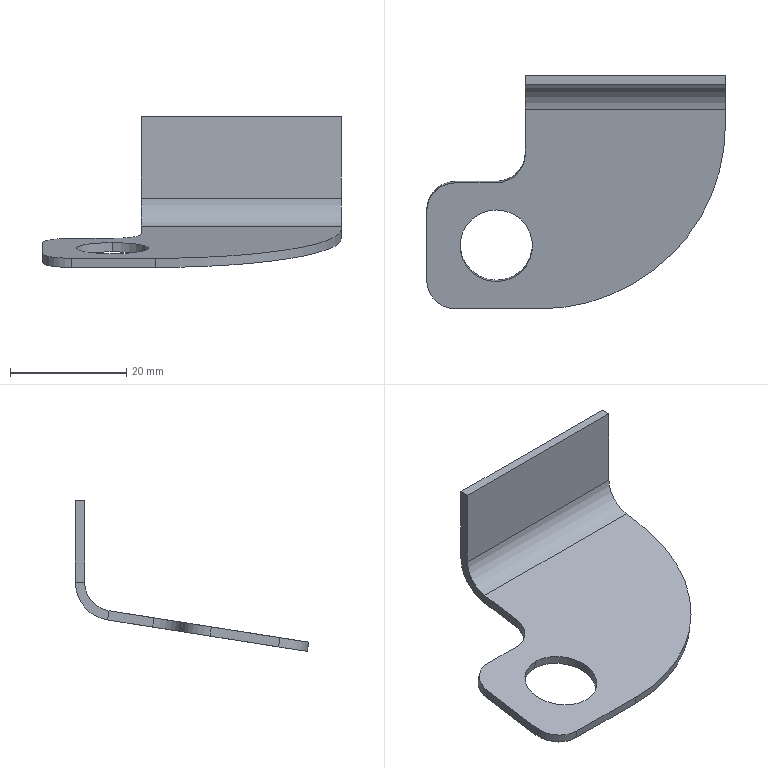Part | SolidWorks | features Fillet 2, ICE 2, FlatPattern 1, SMBaseFlange 1, SheetMetal 1 | 1 solid | 22 faces | box 51.5 x 40.249 x 26 mm | volume 3195 mm3 | plane 14 | cylinder 8 | commonest cylinder face diameters 10 x4 12.5 x2 13.2 x1 64 x1
STEP:
#1=CARTESIAN_POINT('',(-39.5,-23.209,-21.736));
#2=VERTEX_POINT('',#1);
#3=CARTESIAN_POINT('',(-39.5,-35.557,-23.68));
#4=VERTEX_POINT('',#3);
#5=CARTESIAN_POINT('',(-39.5,-29.383,-22.708));
#6=DIRECTION('',(0.,-0.1556,0.9878));
#7=DIRECTION('',(0.,-0.9878,-0.1556));
#8=AXIS2_PLACEMENT_3D('',#5,#6,#7);
#9=CIRCLE('',#8,6.25);
#10=EDGE_CURVE('',#2,#4,#9,.T.);
#11=ORIENTED_EDGE('',*,*,#10,.T.);
#12=CARTESIAN_POINT('',(-39.5,-35.308,-25.261));
#13=VERTEX_POINT('',#12);
#14=CARTESIAN_POINT('',(-39.5,-36.864,-15.383));
#15=DIRECTION('',(0.,0.1556,-0.9878));
#16=VECTOR('',#15,1000.);
#17=LINE('',#14,#16);
#18=EDGE_CURVE('',#4,#13,#17,.T.);
#19=ORIENTED_EDGE('',*,*,#18,.T.);
#20=CARTESIAN_POINT('',(-39.5,-22.96,-23.316));
#21=VERTEX_POINT('',#20);
#22=CARTESIAN_POINT('',(-39.5,-29.134,-24.289));
#23=DIRECTION('',(0.,0.1556,-0.9878));
#24=DIRECTION('',(0.,0.9878,0.1556));
#25=AXIS2_PLACEMENT_3D('',#22,#23,#24);
#26=CIRCLE('',#25,6.25);
#27=EDGE_CURVE('',#13,#21,#26,.T.);
#28=ORIENTED_EDGE('',*,*,#27,.T.);
#29=CARTESIAN_POINT('',(-39.5,-24.516,-13.438));
#30=DIRECTION('',(0.,0.1556,-0.9878));
#31=VECTOR('',#30,1000.);
#32=LINE('',#29,#31);
#33=EDGE_CURVE('',#2,#21,#32,.T.);
#34=ORIENTED_EDGE('',*,*,#33,.F.);
#35=EDGE_LOOP('',(#11,#19,#28,#34));
#36=FACE_OUTER_BOUND('',#35,.T.);
#37=CARTESIAN_POINT('',(-39.5,-30.69,-14.41));
#38=DIRECTION('',(0.,0.1556,-0.9878));
#39=DIRECTION('',(0.,0.9878,0.1556));
#40=AXIS2_PLACEMENT_3D('',#37,#38,#39);
#41=CYLINDRICAL_SURFACE('',#40,6.25);
#42=ADVANCED_FACE('',(#36),#41,.F.);
#43=CARTESIAN_POINT('',(-34.5,0.,-14.058));
#44=VERTEX_POINT('',#43);
#45=CARTESIAN_POINT('',(-34.5,0.,0.));
#46=VERTEX_POINT('',#45);
#47=CARTESIAN_POINT('',(-34.5,0.,0.));
#48=DIRECTION('',(0.,0.,1.));
#49=VECTOR('',#48,1000.);
#50=LINE('',#47,#49);
#51=EDGE_CURVE('',#44,#46,#50,.T.);
#52=ORIENTED_EDGE('',*,*,#51,.F.);
#53=CARTESIAN_POINT('',(-34.5,-1.6,-14.058));
#54=VERTEX_POINT('',#53);
#55=CARTESIAN_POINT('',(-34.5,0.,-14.058));
#56=DIRECTION('',(0.,-1.,0.));
#57=VECTOR('',#56,1000.);
#58=LINE('',#55,#57);
#59=EDGE_CURVE('',#44,#54,#58,.T.);
#60=ORIENTED_EDGE('',*,*,#59,.T.);
#61=CARTESIAN_POINT('',(-34.5,-1.6,0.));
#62=VERTEX_POINT('',#61);
#63=CARTESIAN_POINT('',(-34.5,-1.6,0.));
#64=DIRECTION('',(0.,0.,1.));
#65=VECTOR('',#64,1000.);
#66=LINE('',#63,#65);
#67=EDGE_CURVE('',#54,#62,#66,.T.);
#68=ORIENTED_EDGE('',*,*,#67,.T.);
#69=CARTESIAN_POINT('',(-34.5,-1.6,0.));
#70=DIRECTION('',(0.,-1.,0.));
#71=VECTOR('',#70,1000.);
#72=LINE('',#69,#71);
#73=EDGE_CURVE('',#46,#62,#72,.T.);
#74=ORIENTED_EDGE('',*,*,#73,.F.);
#75=EDGE_LOOP('',(#52,#60,#68,#74));
#76=FACE_OUTER_BOUND('',#75,.T.);
#77=CARTESIAN_POINT('',(-34.5,1.435,-115.54));
#78=DIRECTION('',(1.,0.,0.));
#79=DIRECTION('',(0.,0.,-1.));
#80=AXIS2_PLACEMENT_3D('',#77,#78,#79);
#81=PLANE('',#80);
#82=ADVANCED_FACE('',(#76),#81,.F.);
#83=CARTESIAN_POINT('',(-34.5,-13.578,-20.219));
#84=VERTEX_POINT('',#83);
#85=CARTESIAN_POINT('',(-34.5,-5.822,-18.997));
#86=VERTEX_POINT('',#85);
#87=CARTESIAN_POINT('',(-34.5,-0.2489,-18.119));
#88=DIRECTION('',(0.,0.9878,0.1556));
#89=VECTOR('',#88,1000.);
#90=LINE('',#87,#89);
#91=EDGE_CURVE('',#84,#86,#90,.T.);
#92=ORIENTED_EDGE('',*,*,#91,.T.);
#93=CARTESIAN_POINT('',(-34.5,-5.573,-20.578));
#94=VERTEX_POINT('',#93);
#95=CARTESIAN_POINT('',(-34.5,-5.822,-18.997));
#96=DIRECTION('',(0.,0.1556,-0.9878));
#97=VECTOR('',#96,1000.);
#98=LINE('',#95,#97);
#99=EDGE_CURVE('',#86,#94,#98,.T.);
#100=ORIENTED_EDGE('',*,*,#99,.T.);
#101=CARTESIAN_POINT('',(-34.5,-13.329,-21.799));
#102=VERTEX_POINT('',#101);
#103=CARTESIAN_POINT('',(-34.5,0.,-19.7));
#104=DIRECTION('',(0.,0.9878,0.1556));
#105=VECTOR('',#104,1000.);
#106=LINE('',#103,#105);
#107=EDGE_CURVE('',#102,#94,#106,.T.);
#108=ORIENTED_EDGE('',*,*,#107,.F.);
#109=CARTESIAN_POINT('',(-34.5,1.435,-115.54));
#110=DIRECTION('',(0.,-0.1556,0.9878));
#111=VECTOR('',#110,1000.);
#112=LINE('',#109,#111);
#113=EDGE_CURVE('',#102,#84,#112,.T.);
#114=ORIENTED_EDGE('',*,*,#113,.T.);
#115=EDGE_LOOP('',(#92,#100,#108,#114));
#116=FACE_OUTER_BOUND('',#115,.T.);
#117=CARTESIAN_POINT('',(-34.5,1.435,-115.54));
#118=DIRECTION('',(1.,0.,0.));
#119=DIRECTION('',(0.,0.,-1.));
#120=AXIS2_PLACEMENT_3D('',#117,#118,#119);
#121=PLANE('',#120);
#122=ADVANCED_FACE('',(#116),#121,.F.);
#123=CARTESIAN_POINT('',(0.,-5.573,-20.578));
#124=VERTEX_POINT('',#123);
#125=CARTESIAN_POINT('',(0.,-5.822,-18.997));
#126=VERTEX_POINT('',#125);
#127=CARTESIAN_POINT('',(0.,-5.573,-20.578));
#128=DIRECTION('',(0.,-0.1556,0.9878));
#129=VECTOR('',#128,1000.);
#130=LINE('',#127,#129);
#131=EDGE_CURVE('',#124,#126,#130,.T.);
#132=ORIENTED_EDGE('',*,*,#131,.F.);
#133=CARTESIAN_POINT('',(0.,0.,-14.058));
#134=VERTEX_POINT('',#133);
#135=CARTESIAN_POINT('',(0.,-6.6,-14.058));
#136=DIRECTION('',(-1.,0.,0.));
#137=DIRECTION('',(0.,0.,-1.));
#138=AXIS2_PLACEMENT_3D('',#135,#136,#137);
#139=CIRCLE('',#138,6.6);
#140=EDGE_CURVE('',#134,#124,#139,.T.);
#141=ORIENTED_EDGE('',*,*,#140,.F.);
#142=CARTESIAN_POINT('',(0.,-1.6,-14.058));
#143=VERTEX_POINT('',#142);
#144=CARTESIAN_POINT('',(0.,-1.6,-14.058));
#145=DIRECTION('',(0.,1.,0.));
#146=VECTOR('',#145,1000.);
#147=LINE('',#144,#146);
#148=EDGE_CURVE('',#143,#134,#147,.T.);
#149=ORIENTED_EDGE('',*,*,#148,.F.);
#150=CARTESIAN_POINT('',(0.,-6.6,-14.058));
#151=DIRECTION('',(-1.,0.,0.));
#152=DIRECTION('',(0.,0.,-1.));
#153=AXIS2_PLACEMENT_3D('',#150,#151,#152);
#154=CIRCLE('',#153,5.);
#155=EDGE_CURVE('',#143,#126,#154,.T.);
#156=ORIENTED_EDGE('',*,*,#155,.T.);
#157=EDGE_LOOP('',(#132,#141,#149,#156));
#158=FACE_OUTER_BOUND('',#157,.T.);
#159=CARTESIAN_POINT('',(0.,-5.573,-20.578));
#160=DIRECTION('',(1.,0.,0.));
#161=DIRECTION('',(0.,0.,-1.));
#162=AXIS2_PLACEMENT_3D('',#159,#160,#161);
#163=PLANE('',#162);
#164=ADVANCED_FACE('',(#158),#163,.T.);
#165=CARTESIAN_POINT('',(0.,-8.639,-19.441));
#166=VERTEX_POINT('',#165);
#167=CARTESIAN_POINT('',(0.,-0.2489,-18.119));
#168=DIRECTION('',(0.,-0.9878,-0.1556));
#169=VECTOR('',#168,1000.);
#170=LINE('',#167,#169);
#171=EDGE_CURVE('',#126,#166,#170,.T.);
#172=ORIENTED_EDGE('',*,*,#171,.T.);
#173=CARTESIAN_POINT('',(0.,-8.39,-21.021));
#174=VERTEX_POINT('',#173);
#175=CARTESIAN_POINT('',(0.,-8.39,-21.021));
#176=DIRECTION('',(0.,0.1556,-0.9878));
#177=VECTOR('',#176,1000.);
#178=LINE('',#175,#177);
#179=EDGE_CURVE('',#166,#174,#178,.T.);
#180=ORIENTED_EDGE('',*,*,#179,.T.);
#181=CARTESIAN_POINT('',(0.,0.,-19.7));
#182=DIRECTION('',(0.,-0.9878,-0.1556));
#183=VECTOR('',#182,1000.);
#184=LINE('',#181,#183);
#185=EDGE_CURVE('',#124,#174,#184,.T.);
#186=ORIENTED_EDGE('',*,*,#185,.F.);
#187=ORIENTED_EDGE('',*,*,#131,.T.);
#188=EDGE_LOOP('',(#172,#180,#186,#187));
#189=FACE_OUTER_BOUND('',#188,.T.);
#190=CARTESIAN_POINT('',(0.,-1.6,-14.058));
#191=DIRECTION('',(1.,0.,0.));
#192=DIRECTION('',(0.,0.,-1.));
#193=AXIS2_PLACEMENT_3D('',#190,#191,#192);
#194=PLANE('',#193);
#195=ADVANCED_FACE('',(#189),#194,.T.);
#196=ORIENTED_EDGE('',*,*,#10,.F.);
#197=CARTESIAN_POINT('',(-39.5,-29.383,-22.708));
#198=DIRECTION('',(0.,-0.1556,0.9878));
#199=DIRECTION('',(0.,-0.9878,-0.1556));
#200=AXIS2_PLACEMENT_3D('',#197,#198,#199);
#201=CIRCLE('',#200,6.25);
#202=EDGE_CURVE('',#4,#2,#201,.T.);
#203=ORIENTED_EDGE('',*,*,#202,.F.);
#204=EDGE_LOOP('',(#196,#203));
#205=FACE_BOUND('',#204,.T.);
#206=CARTESIAN_POINT('',(-46.5,-40.249,-24.419));
#207=VERTEX_POINT('',#206);
#208=CARTESIAN_POINT('',(-32.,-40.249,-24.419));
#209=VERTEX_POINT('',#208);
#210=CARTESIAN_POINT('',(-51.5,-40.249,-24.419));
#211=DIRECTION('',(1.,0.,0.));
#212=VECTOR('',#211,1000.);
#213=LINE('',#210,#212);
#214=EDGE_CURVE('',#207,#209,#213,.T.);
#215=ORIENTED_EDGE('',*,*,#214,.T.);
#216=CARTESIAN_POINT('',(-32.,-8.639,-19.441));
#217=DIRECTION('',(0.,-0.1556,0.9878));
#218=DIRECTION('',(0.,-0.9878,-0.1556));
#219=AXIS2_PLACEMENT_3D('',#216,#217,#218);
#220=CIRCLE('',#219,32.);
#221=EDGE_CURVE('',#209,#166,#220,.T.);
#222=ORIENTED_EDGE('',*,*,#221,.T.);
#223=ORIENTED_EDGE('',*,*,#171,.F.);
#224=CARTESIAN_POINT('',(-51.5,-5.822,-18.997));
#225=DIRECTION('',(1.,0.,0.));
#226=VECTOR('',#225,1000.);
#227=LINE('',#224,#226);
#228=EDGE_CURVE('',#86,#126,#227,.T.);
#229=ORIENTED_EDGE('',*,*,#228,.F.);
#230=ORIENTED_EDGE('',*,*,#91,.F.);
#231=CARTESIAN_POINT('',(-39.5,-18.517,-20.997));
#232=VERTEX_POINT('',#231);
#233=CARTESIAN_POINT('',(-39.5,-13.578,-20.219));
#234=DIRECTION('',(0.,-0.1556,0.9878));
#235=DIRECTION('',(0.,-0.9878,-0.1556));
#236=AXIS2_PLACEMENT_3D('',#233,#234,#235);
#237=CIRCLE('',#236,5.);
#238=EDGE_CURVE('',#232,#84,#237,.T.);
#239=ORIENTED_EDGE('',*,*,#238,.F.);
#240=CARTESIAN_POINT('',(-46.5,-18.517,-20.997));
#241=VERTEX_POINT('',#240);
#242=CARTESIAN_POINT('',(-51.5,-18.517,-20.997));
#243=DIRECTION('',(1.,0.,0.));
#244=VECTOR('',#243,1000.);
#245=LINE('',#242,#244);
#246=EDGE_CURVE('',#241,#232,#245,.T.);
#247=ORIENTED_EDGE('',*,*,#246,.F.);
#248=CARTESIAN_POINT('',(-51.5,-23.456,-21.775));
#249=VERTEX_POINT('',#248);
#250=CARTESIAN_POINT('',(-46.5,-23.456,-21.775));
#251=DIRECTION('',(0.,-0.1556,0.9878));
#252=DIRECTION('',(0.,-0.9878,-0.1556));
#253=AXIS2_PLACEMENT_3D('',#250,#251,#252);
#254=CIRCLE('',#253,5.);
#255=EDGE_CURVE('',#241,#249,#254,.T.);
#256=ORIENTED_EDGE('',*,*,#255,.T.);
#257=CARTESIAN_POINT('',(-51.5,-35.31,-23.642));
#258=VERTEX_POINT('',#257);
#259=CARTESIAN_POINT('',(-51.5,-0.2489,-18.119));
#260=DIRECTION('',(0.,-0.9878,-0.1556));
#261=VECTOR('',#260,1000.);
#262=LINE('',#259,#261);
#263=EDGE_CURVE('',#249,#258,#262,.T.);
#264=ORIENTED_EDGE('',*,*,#263,.T.);
#265=CARTESIAN_POINT('',(-46.5,-35.31,-23.642));
#266=DIRECTION('',(0.,-0.1556,0.9878));
#267=DIRECTION('',(0.,-0.9878,-0.1556));
#268=AXIS2_PLACEMENT_3D('',#265,#266,#267);
#269=CIRCLE('',#268,5.);
#270=EDGE_CURVE('',#258,#207,#269,.T.);
#271=ORIENTED_EDGE('',*,*,#270,.T.);
#272=EDGE_LOOP('',(#215,#222,#223,#229,#230,#239,#247,#256,#264,#271));
#273=FACE_OUTER_BOUND('',#272,.T.);
#274=CARTESIAN_POINT('',(-51.5,-0.2489,-18.119));
#275=DIRECTION('',(0.,-0.1556,0.9878));
#276=DIRECTION('',(0.,-0.9878,-0.1556));
#277=AXIS2_PLACEMENT_3D('',#274,#275,#276);
#278=PLANE('',#277);
#279=ADVANCED_FACE('',(#205,#273),#278,.T.);
#280=CARTESIAN_POINT('',(-34.5,-6.6,-14.058));
#281=DIRECTION('',(1.,0.,0.));
#282=DIRECTION('',(0.,0.,-1.));
#283=AXIS2_PLACEMENT_3D('',#280,#281,#282);
#284=CIRCLE('',#283,5.);
#285=EDGE_CURVE('',#86,#54,#284,.T.);
#286=ORIENTED_EDGE('',*,*,#285,.F.);
#287=ORIENTED_EDGE('',*,*,#228,.T.);
#288=ORIENTED_EDGE('',*,*,#155,.F.);
#289=CARTESIAN_POINT('',(-51.5,-1.6,-14.058));
#290=DIRECTION('',(1.,0.,0.));
#291=VECTOR('',#290,1000.);
#292=LINE('',#289,#291);
#293=EDGE_CURVE('',#54,#143,#292,.T.);
#294=ORIENTED_EDGE('',*,*,#293,.F.);
#295=EDGE_LOOP('',(#286,#287,#288,#294));
#296=FACE_OUTER_BOUND('',#295,.T.);
#297=CARTESIAN_POINT('',(-51.5,-6.6,-14.058));
#298=DIRECTION('',(1.,0.,0.));
#299=DIRECTION('',(0.,0.,-1.));
#300=AXIS2_PLACEMENT_3D('',#297,#298,#299);
#301=CYLINDRICAL_SURFACE('',#300,5.);
#302=ADVANCED_FACE('',(#296),#301,.F.);
#303=ORIENTED_EDGE('',*,*,#67,.F.);
#304=ORIENTED_EDGE('',*,*,#293,.T.);
#305=CARTESIAN_POINT('',(0.,-1.6,0.));
#306=VERTEX_POINT('',#305);
#307=CARTESIAN_POINT('',(0.,-1.6,0.));
#308=DIRECTION('',(0.,0.,-1.));
#309=VECTOR('',#308,1000.);
#310=LINE('',#307,#309);
#311=EDGE_CURVE('',#306,#143,#310,.T.);
#312=ORIENTED_EDGE('',*,*,#311,.F.);
#313=CARTESIAN_POINT('',(-51.5,-1.6,0.));
#314=DIRECTION('',(1.,0.,0.));
#315=VECTOR('',#314,1000.);
#316=LINE('',#313,#315);
#317=EDGE_CURVE('',#62,#306,#316,.T.);
#318=ORIENTED_EDGE('',*,*,#317,.F.);
#319=EDGE_LOOP('',(#303,#304,#312,#318));
#320=FACE_OUTER_BOUND('',#319,.T.);
#321=CARTESIAN_POINT('',(-51.5,-1.6,0.));
#322=DIRECTION('',(0.,-1.,0.));
#323=DIRECTION('',(0.,0.,-1.));
#324=AXIS2_PLACEMENT_3D('',#321,#322,#323);
#325=PLANE('',#324);
#326=ADVANCED_FACE('',(#320),#325,.T.);
#327=CARTESIAN_POINT('',(0.,0.,0.));
#328=VERTEX_POINT('',#327);
#329=CARTESIAN_POINT('',(-51.5,0.,0.));
#330=DIRECTION('',(1.,0.,0.));
#331=VECTOR('',#330,1000.);
#332=LINE('',#329,#331);
#333=EDGE_CURVE('',#46,#328,#332,.T.);
#334=ORIENTED_EDGE('',*,*,#333,.F.);
#335=ORIENTED_EDGE('',*,*,#73,.T.);
#336=ORIENTED_EDGE('',*,*,#317,.T.);
#337=CARTESIAN_POINT('',(0.,-1.6,0.));
#338=DIRECTION('',(0.,1.,0.));
#339=VECTOR('',#338,1000.);
#340=LINE('',#337,#339);
#341=EDGE_CURVE('',#306,#328,#340,.T.);
#342=ORIENTED_EDGE('',*,*,#341,.T.);
#343=EDGE_LOOP('',(#334,#335,#336,#342));
#344=FACE_OUTER_BOUND('',#343,.T.);
#345=CARTESIAN_POINT('',(-51.5,-1.6,0.));
#346=DIRECTION('',(0.,0.,-1.));
#347=DIRECTION('',(-1.,0.,0.));
#348=AXIS2_PLACEMENT_3D('',#345,#346,#347);
#349=PLANE('',#348);
#350=ADVANCED_FACE('',(#344),#349,.F.);
#351=CARTESIAN_POINT('',(-51.5,0.,-14.058));
#352=DIRECTION('',(1.,0.,0.));
#353=VECTOR('',#352,1000.);
#354=LINE('',#351,#353);
#355=EDGE_CURVE('',#44,#134,#354,.T.);
#356=ORIENTED_EDGE('',*,*,#355,.F.);
#357=ORIENTED_EDGE('',*,*,#51,.T.);
#358=ORIENTED_EDGE('',*,*,#333,.T.);
#359=CARTESIAN_POINT('',(0.,0.,0.));
#360=DIRECTION('',(0.,0.,-1.));
#361=VECTOR('',#360,1000.);
#362=LINE('',#359,#361);
#363=EDGE_CURVE('',#328,#134,#362,.T.);
#364=ORIENTED_EDGE('',*,*,#363,.T.);
#365=EDGE_LOOP('',(#356,#357,#358,#364));
#366=FACE_OUTER_BOUND('',#365,.T.);
#367=CARTESIAN_POINT('',(-51.5,0.,0.));
#368=DIRECTION('',(0.,-1.,0.));
#369=DIRECTION('',(0.,0.,-1.));
#370=AXIS2_PLACEMENT_3D('',#367,#368,#369);
#371=PLANE('',#370);
#372=ADVANCED_FACE('',(#366),#371,.F.);
#373=CARTESIAN_POINT('',(-51.5,-5.573,-20.578));
#374=DIRECTION('',(1.,0.,0.));
#375=VECTOR('',#374,1000.);
#376=LINE('',#373,#375);
#377=EDGE_CURVE('',#94,#124,#376,.T.);
#378=ORIENTED_EDGE('',*,*,#377,.F.);
#379=CARTESIAN_POINT('',(-34.5,-6.6,-14.058));
#380=DIRECTION('',(1.,0.,0.));
#381=DIRECTION('',(0.,0.,-1.));
#382=AXIS2_PLACEMENT_3D('',#379,#380,#381);
#383=CIRCLE('',#382,6.6);
#384=EDGE_CURVE('',#94,#44,#383,.T.);
#385=ORIENTED_EDGE('',*,*,#384,.T.);
#386=ORIENTED_EDGE('',*,*,#355,.T.);
#387=ORIENTED_EDGE('',*,*,#140,.T.);
#388=EDGE_LOOP('',(#378,#385,#386,#387));
#389=FACE_OUTER_BOUND('',#388,.T.);
#390=CARTESIAN_POINT('',(-51.5,-6.6,-14.058));
#391=DIRECTION('',(1.,0.,0.));
#392=DIRECTION('',(0.,0.,-1.));
#393=AXIS2_PLACEMENT_3D('',#390,#391,#392);
#394=CYLINDRICAL_SURFACE('',#393,6.6);
#395=ADVANCED_FACE('',(#389),#394,.T.);
#396=CARTESIAN_POINT('',(-39.5,-29.134,-24.289));
#397=DIRECTION('',(0.,0.1556,-0.9878));
#398=DIRECTION('',(0.,0.9878,0.1556));
#399=AXIS2_PLACEMENT_3D('',#396,#397,#398);
#400=CIRCLE('',#399,6.25);
#401=EDGE_CURVE('',#21,#13,#400,.T.);
#402=ORIENTED_EDGE('',*,*,#401,.F.);
#403=ORIENTED_EDGE('',*,*,#27,.F.);
#404=EDGE_LOOP('',(#402,#403));
#405=FACE_BOUND('',#404,.T.);
#406=ORIENTED_EDGE('',*,*,#185,.T.);
#407=CARTESIAN_POINT('',(-32.,-40.,-26.));
#408=VERTEX_POINT('',#407);
#409=CARTESIAN_POINT('',(-32.,-8.39,-21.021));
#410=DIRECTION('',(0.,0.1556,-0.9878));
#411=DIRECTION('',(0.,-0.9878,-0.1556));
#412=AXIS2_PLACEMENT_3D('',#409,#410,#411);
#413=CIRCLE('',#412,32.);
#414=EDGE_CURVE('',#174,#408,#413,.T.);
#415=ORIENTED_EDGE('',*,*,#414,.T.);
#416=CARTESIAN_POINT('',(-46.5,-40.,-26.));
#417=VERTEX_POINT('',#416);
#418=CARTESIAN_POINT('',(-51.5,-40.,-26.));
#419=DIRECTION('',(1.,0.,0.));
#420=VECTOR('',#419,1000.);
#421=LINE('',#418,#420);
#422=EDGE_CURVE('',#417,#408,#421,.T.);
#423=ORIENTED_EDGE('',*,*,#422,.F.);
#424=CARTESIAN_POINT('',(-51.5,-35.061,-25.222));
#425=VERTEX_POINT('',#424);
#426=CARTESIAN_POINT('',(-46.5,-35.061,-25.222));
#427=DIRECTION('',(0.,0.1556,-0.9878));
#428=DIRECTION('',(0.,-0.9878,-0.1556));
#429=AXIS2_PLACEMENT_3D('',#426,#427,#428);
#430=CIRCLE('',#429,5.);
#431=EDGE_CURVE('',#417,#425,#430,.T.);
#432=ORIENTED_EDGE('',*,*,#431,.T.);
#433=CARTESIAN_POINT('',(-51.5,-23.207,-23.355));
#434=VERTEX_POINT('',#433);
#435=CARTESIAN_POINT('',(-51.5,0.,-19.7));
#436=DIRECTION('',(0.,-0.9878,-0.1556));
#437=VECTOR('',#436,1000.);
#438=LINE('',#435,#437);
#439=EDGE_CURVE('',#434,#425,#438,.T.);
#440=ORIENTED_EDGE('',*,*,#439,.F.);
#441=CARTESIAN_POINT('',(-46.5,-18.268,-22.577));
#442=VERTEX_POINT('',#441);
#443=CARTESIAN_POINT('',(-46.5,-23.207,-23.355));
#444=DIRECTION('',(0.,0.1556,-0.9878));
#445=DIRECTION('',(0.,-0.9878,-0.1556));
#446=AXIS2_PLACEMENT_3D('',#443,#444,#445);
#447=CIRCLE('',#446,5.);
#448=EDGE_CURVE('',#434,#442,#447,.T.);
#449=ORIENTED_EDGE('',*,*,#448,.T.);
#450=CARTESIAN_POINT('',(-39.5,-18.268,-22.577));
#451=VERTEX_POINT('',#450);
#452=CARTESIAN_POINT('',(-51.5,-18.268,-22.577));
#453=DIRECTION('',(1.,0.,0.));
#454=VECTOR('',#453,1000.);
#455=LINE('',#452,#454);
#456=EDGE_CURVE('',#442,#451,#455,.T.);
#457=ORIENTED_EDGE('',*,*,#456,.T.);
#458=CARTESIAN_POINT('',(-39.5,-13.329,-21.799));
#459=DIRECTION('',(0.,-0.1556,0.9878));
#460=DIRECTION('',(0.,-0.9878,-0.1556));
#461=AXIS2_PLACEMENT_3D('',#458,#459,#460);
#462=CIRCLE('',#461,5.);
#463=EDGE_CURVE('',#451,#102,#462,.T.);
#464=ORIENTED_EDGE('',*,*,#463,.T.);
#465=ORIENTED_EDGE('',*,*,#107,.T.);
#466=ORIENTED_EDGE('',*,*,#377,.T.);
#467=EDGE_LOOP('',(#406,#415,#423,#432,#440,#449,#457,#464,#465,#466));
#468=FACE_OUTER_BOUND('',#467,.T.);
#469=CARTESIAN_POINT('',(-51.5,0.,-19.7));
#470=DIRECTION('',(0.,-0.1556,0.9878));
#471=DIRECTION('',(0.,-0.9878,-0.1556));
#472=AXIS2_PLACEMENT_3D('',#469,#470,#471);
#473=PLANE('',#472);
#474=ADVANCED_FACE('',(#405,#468),#473,.F.);
#475=ORIENTED_EDGE('',*,*,#422,.T.);
#476=CARTESIAN_POINT('',(-32.,-40.249,-24.419));
#477=DIRECTION('',(0.,-0.1556,0.9878));
#478=VECTOR('',#477,1000.);
#479=LINE('',#476,#478);
#480=EDGE_CURVE('',#408,#209,#479,.T.);
#481=ORIENTED_EDGE('',*,*,#480,.T.);
#482=ORIENTED_EDGE('',*,*,#214,.F.);
#483=CARTESIAN_POINT('',(-46.5,-40.,-26.));
#484=DIRECTION('',(0.,0.1556,-0.9878));
#485=VECTOR('',#484,1000.);
#486=LINE('',#483,#485);
#487=EDGE_CURVE('',#207,#417,#486,.T.);
#488=ORIENTED_EDGE('',*,*,#487,.T.);
#489=EDGE_LOOP('',(#475,#481,#482,#488));
#490=FACE_OUTER_BOUND('',#489,.T.);
#491=CARTESIAN_POINT('',(-51.5,-40.,-26.));
#492=DIRECTION('',(0.,0.9878,0.1556));
#493=DIRECTION('',(0.,-0.1556,0.9878));
#494=AXIS2_PLACEMENT_3D('',#491,#492,#493);
#495=PLANE('',#494);
#496=ADVANCED_FACE('',(#490),#495,.F.);
#497=ORIENTED_EDGE('',*,*,#439,.T.);
#498=CARTESIAN_POINT('',(-51.5,-36.088,-18.702));
#499=DIRECTION('',(0.,-0.1556,0.9878));
#500=VECTOR('',#499,1000.);
#501=LINE('',#498,#500);
#502=EDGE_CURVE('',#425,#258,#501,.T.);
#503=ORIENTED_EDGE('',*,*,#502,.T.);
#504=ORIENTED_EDGE('',*,*,#263,.F.);
#505=CARTESIAN_POINT('',(-51.5,-24.234,-16.835));
#506=DIRECTION('',(0.,0.1556,-0.9878));
#507=VECTOR('',#506,1000.);
#508=LINE('',#505,#507);
#509=EDGE_CURVE('',#249,#434,#508,.T.);
#510=ORIENTED_EDGE('',*,*,#509,.T.);
#511=EDGE_LOOP('',(#497,#503,#504,#510));
#512=FACE_OUTER_BOUND('',#511,.T.);
#513=CARTESIAN_POINT('',(-51.5,-6.6,-14.058));
#514=DIRECTION('',(1.,0.,0.));
#515=DIRECTION('',(0.,0.,-1.));
#516=AXIS2_PLACEMENT_3D('',#513,#514,#515);
#517=PLANE('',#516);
#518=ADVANCED_FACE('',(#512),#517,.F.);
#519=ORIENTED_EDGE('',*,*,#311,.T.);
#520=ORIENTED_EDGE('',*,*,#148,.T.);
#521=ORIENTED_EDGE('',*,*,#363,.F.);
#522=ORIENTED_EDGE('',*,*,#341,.F.);
#523=EDGE_LOOP('',(#519,#520,#521,#522));
#524=FACE_OUTER_BOUND('',#523,.T.);
#525=CARTESIAN_POINT('',(0.,-6.6,-14.058));
#526=DIRECTION('',(1.,0.,0.));
#527=DIRECTION('',(0.,0.,-1.));
#528=AXIS2_PLACEMENT_3D('',#525,#526,#527);
#529=PLANE('',#528);
#530=ADVANCED_FACE('',(#524),#529,.T.);
#531=CARTESIAN_POINT('',(-39.5,-3.504,-116.318));
#532=DIRECTION('',(0.,-0.1556,0.9878));
#533=VECTOR('',#532,1000.);
#534=LINE('',#531,#533);
#535=EDGE_CURVE('',#451,#232,#534,.T.);
#536=ORIENTED_EDGE('',*,*,#535,.T.);
#537=ORIENTED_EDGE('',*,*,#238,.T.);
#538=ORIENTED_EDGE('',*,*,#113,.F.);
#539=ORIENTED_EDGE('',*,*,#463,.F.);
#540=EDGE_LOOP('',(#536,#537,#538,#539));
#541=FACE_OUTER_BOUND('',#540,.T.);
#542=CARTESIAN_POINT('',(-39.5,1.435,-115.54));
#543=DIRECTION('',(0.,-0.1556,0.9878));
#544=DIRECTION('',(0.,-0.9878,-0.1556));
#545=AXIS2_PLACEMENT_3D('',#542,#543,#544);
#546=CYLINDRICAL_SURFACE('',#545,5.);
#547=ADVANCED_FACE('',(#541),#546,.F.);
#548=ORIENTED_EDGE('',*,*,#59,.F.);
#549=ORIENTED_EDGE('',*,*,#384,.F.);
#550=ORIENTED_EDGE('',*,*,#99,.F.);
#551=ORIENTED_EDGE('',*,*,#285,.T.);
#552=EDGE_LOOP('',(#548,#549,#550,#551));
#553=FACE_OUTER_BOUND('',#552,.T.);
#554=CARTESIAN_POINT('',(-34.5,1.435,-115.54));
#555=DIRECTION('',(1.,0.,0.));
#556=DIRECTION('',(0.,0.,-1.));
#557=AXIS2_PLACEMENT_3D('',#554,#555,#556);
#558=PLANE('',#557);
#559=ADVANCED_FACE('',(#553),#558,.F.);
#560=ORIENTED_EDGE('',*,*,#456,.F.);
#561=CARTESIAN_POINT('',(-46.5,-3.504,-116.318));
#562=DIRECTION('',(0.,-0.1556,0.9878));
#563=VECTOR('',#562,1000.);
#564=LINE('',#561,#563);
#565=EDGE_CURVE('',#442,#241,#564,.T.);
#566=ORIENTED_EDGE('',*,*,#565,.T.);
#567=ORIENTED_EDGE('',*,*,#246,.T.);
#568=ORIENTED_EDGE('',*,*,#535,.F.);
#569=EDGE_LOOP('',(#560,#566,#567,#568));
#570=FACE_OUTER_BOUND('',#569,.T.);
#571=CARTESIAN_POINT('',(-51.5,-3.504,-116.318));
#572=DIRECTION('',(0.,-0.9878,-0.1556));
#573=DIRECTION('',(0.,0.1556,-0.9878));
#574=AXIS2_PLACEMENT_3D('',#571,#572,#573);
#575=PLANE('',#574);
#576=ADVANCED_FACE('',(#570),#575,.F.);
#577=ORIENTED_EDGE('',*,*,#431,.F.);
#578=ORIENTED_EDGE('',*,*,#487,.F.);
#579=ORIENTED_EDGE('',*,*,#270,.F.);
#580=ORIENTED_EDGE('',*,*,#502,.F.);
#581=EDGE_LOOP('',(#577,#578,#579,#580));
#582=FACE_OUTER_BOUND('',#581,.T.);
#583=CARTESIAN_POINT('',(-46.5,-36.088,-18.702));
#584=DIRECTION('',(0.,-0.1556,0.9878));
#585=DIRECTION('',(0.,-0.9878,-0.1556));
#586=AXIS2_PLACEMENT_3D('',#583,#584,#585);
#587=CYLINDRICAL_SURFACE('',#586,5.);
#588=ADVANCED_FACE('',(#582),#587,.T.);
#589=ORIENTED_EDGE('',*,*,#255,.F.);
#590=ORIENTED_EDGE('',*,*,#565,.F.);
#591=ORIENTED_EDGE('',*,*,#448,.F.);
#592=ORIENTED_EDGE('',*,*,#509,.F.);
#593=EDGE_LOOP('',(#589,#590,#591,#592));
#594=FACE_OUTER_BOUND('',#593,.T.);
#595=CARTESIAN_POINT('',(-46.5,-24.234,-16.835));
#596=DIRECTION('',(0.,0.1556,-0.9878));
#597=DIRECTION('',(0.,0.9878,0.1556));
#598=AXIS2_PLACEMENT_3D('',#595,#596,#597);
#599=CYLINDRICAL_SURFACE('',#598,5.);
#600=ADVANCED_FACE('',(#594),#599,.T.);
#601=ORIENTED_EDGE('',*,*,#414,.F.);
#602=ORIENTED_EDGE('',*,*,#179,.F.);
#603=ORIENTED_EDGE('',*,*,#221,.F.);
#604=ORIENTED_EDGE('',*,*,#480,.F.);
#605=EDGE_LOOP('',(#601,#602,#603,#604));
#606=FACE_OUTER_BOUND('',#605,.T.);
#607=CARTESIAN_POINT('',(-32.,-8.39,-21.021));
#608=DIRECTION('',(0.,0.1556,-0.9878));
#609=DIRECTION('',(0.,0.9878,0.1556));
#610=AXIS2_PLACEMENT_3D('',#607,#608,#609);
#611=CYLINDRICAL_SURFACE('',#610,32.);
#612=ADVANCED_FACE('',(#606),#611,.T.);
#613=ORIENTED_EDGE('',*,*,#18,.F.);
#614=ORIENTED_EDGE('',*,*,#202,.T.);
#615=ORIENTED_EDGE('',*,*,#33,.T.);
#616=ORIENTED_EDGE('',*,*,#401,.T.);
#617=EDGE_LOOP('',(#613,#614,#615,#616));
#618=FACE_OUTER_BOUND('',#617,.T.);
#619=CARTESIAN_POINT('',(-39.5,-30.69,-14.41));
#620=DIRECTION('',(0.,0.1556,-0.9878));
#621=DIRECTION('',(0.,0.9878,0.1556));
#622=AXIS2_PLACEMENT_3D('',#619,#620,#621);
#623=CYLINDRICAL_SURFACE('',#622,6.25);
#624=ADVANCED_FACE('',(#618),#623,.F.);
#625=CLOSED_SHELL('',(#42,#82,#122,#164,#195,#279,#302,#326,#350,#372,#395,#474,#496,#518,#530,#547,#559,#576,#588,#600,#612,#624));
#626=MANIFOLD_SOLID_BREP('',#625);
#627=CARTESIAN_POINT('',(0.,0.,0.));
#628=DIRECTION('',(0.,0.,1.));
#629=DIRECTION('',(1.,0.,0.));
#630=AXIS2_PLACEMENT_3D('',#627,#628,#629);
#631=(LENGTH_UNIT()NAMED_UNIT(*)SI_UNIT(.MILLI.,.METRE.));
#632=UNCERTAINTY_MEASURE_WITH_UNIT(LENGTH_MEASURE(0.00001),#631,'','');
#633=(NAMED_UNIT(*)PLANE_ANGLE_UNIT()SI_UNIT($,.RADIAN.));
#634=(NAMED_UNIT(*)SI_UNIT($,.STERADIAN.)SOLID_ANGLE_UNIT());
#635=(GEOMETRIC_REPRESENTATION_CONTEXT(3)GLOBAL_UNCERTAINTY_ASSIGNED_CONTEXT((#632))GLOBAL_UNIT_ASSIGNED_CONTEXT((#631,#633,#634))REPRESENTATION_CONTEXT('',''));
#636=ADVANCED_BREP_SHAPE_REPRESENTATION('',(#626,#630),#635);